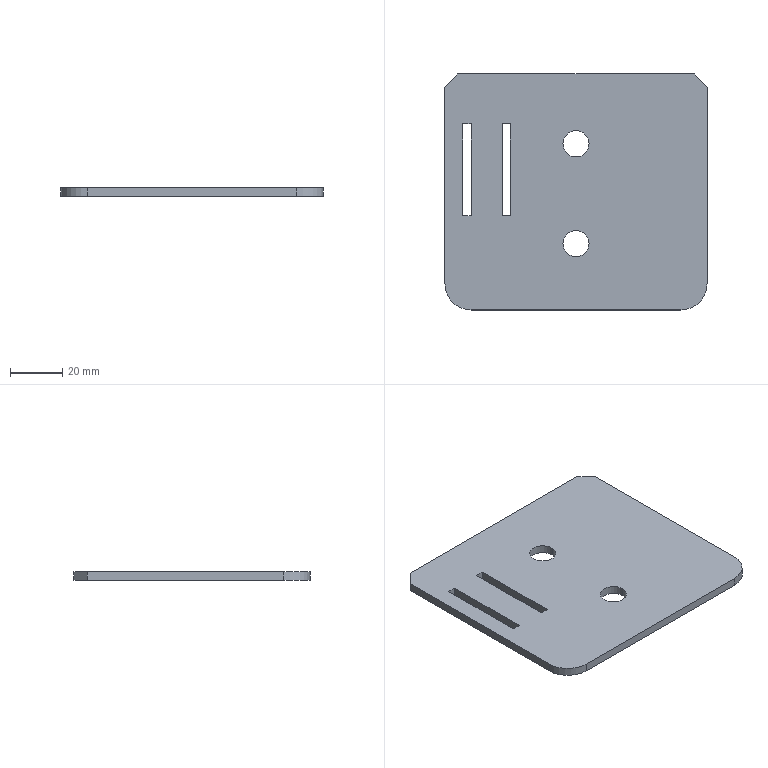Part | SolidWorks | features FlatPattern 1, SMBaseFlange 1, SheetMetal 1 | 1 solid | 22 faces | box 100 x 90 x 3.2 mm | volume 27363 mm3 | plane 16 | cylinder 6 | commonest cylinder face diameters 10 x4 20 x2
STEP:
#1=CARTESIAN_POINT('',(-190.,439.179,3.2));
#2=VERTEX_POINT('',#1);
#3=CARTESIAN_POINT('',(-180.,439.179,3.2));
#4=VERTEX_POINT('',#3);
#5=CARTESIAN_POINT('',(-185.,439.179,3.2));
#6=DIRECTION('',(0.,0.,1.));
#7=DIRECTION('',(1.,0.,0.));
#8=AXIS2_PLACEMENT_3D('',#5,#6,#7);
#9=CIRCLE('',#8,5.);
#10=EDGE_CURVE('',#2,#4,#9,.T.);
#11=ORIENTED_EDGE('',*,*,#10,.T.);
#12=CARTESIAN_POINT('',(-180.,439.179,0.));
#13=VERTEX_POINT('',#12);
#14=CARTESIAN_POINT('',(-180.,439.179,3.2));
#15=DIRECTION('',(0.,0.,-1.));
#16=VECTOR('',#15,1000.);
#17=LINE('',#14,#16);
#18=EDGE_CURVE('',#4,#13,#17,.T.);
#19=ORIENTED_EDGE('',*,*,#18,.T.);
#20=CARTESIAN_POINT('',(-190.,439.179,0.));
#21=VERTEX_POINT('',#20);
#22=CARTESIAN_POINT('',(-185.,439.179,0.));
#23=DIRECTION('',(0.,0.,1.));
#24=DIRECTION('',(1.,0.,0.));
#25=AXIS2_PLACEMENT_3D('',#22,#23,#24);
#26=CIRCLE('',#25,5.);
#27=EDGE_CURVE('',#21,#13,#26,.T.);
#28=ORIENTED_EDGE('',*,*,#27,.F.);
#29=CARTESIAN_POINT('',(-190.,439.179,3.2));
#30=DIRECTION('',(0.,0.,-1.));
#31=VECTOR('',#30,1000.);
#32=LINE('',#29,#31);
#33=EDGE_CURVE('',#2,#21,#32,.T.);
#34=ORIENTED_EDGE('',*,*,#33,.F.);
#35=EDGE_LOOP('',(#11,#19,#28,#34));
#36=FACE_OUTER_BOUND('',#35,.T.);
#37=CARTESIAN_POINT('',(-185.,439.179,3.2));
#38=DIRECTION('',(0.,0.,-1.));
#39=DIRECTION('',(-1.,0.,0.));
#40=AXIS2_PLACEMENT_3D('',#37,#38,#39);
#41=CYLINDRICAL_SURFACE('',#40,5.);
#42=ADVANCED_FACE('',(#36),#41,.F.);
#43=CARTESIAN_POINT('',(-190.,477.279,3.2));
#44=VERTEX_POINT('',#43);
#45=CARTESIAN_POINT('',(-180.,477.279,3.2));
#46=VERTEX_POINT('',#45);
#47=CARTESIAN_POINT('',(-185.,477.279,3.2));
#48=DIRECTION('',(0.,0.,1.));
#49=DIRECTION('',(1.,0.,0.));
#50=AXIS2_PLACEMENT_3D('',#47,#48,#49);
#51=CIRCLE('',#50,5.);
#52=EDGE_CURVE('',#44,#46,#51,.T.);
#53=ORIENTED_EDGE('',*,*,#52,.T.);
#54=CARTESIAN_POINT('',(-180.,477.279,0.));
#55=VERTEX_POINT('',#54);
#56=CARTESIAN_POINT('',(-180.,477.279,3.2));
#57=DIRECTION('',(0.,0.,-1.));
#58=VECTOR('',#57,1000.);
#59=LINE('',#56,#58);
#60=EDGE_CURVE('',#46,#55,#59,.T.);
#61=ORIENTED_EDGE('',*,*,#60,.T.);
#62=CARTESIAN_POINT('',(-190.,477.279,0.));
#63=VERTEX_POINT('',#62);
#64=CARTESIAN_POINT('',(-185.,477.279,0.));
#65=DIRECTION('',(0.,0.,1.));
#66=DIRECTION('',(1.,0.,0.));
#67=AXIS2_PLACEMENT_3D('',#64,#65,#66);
#68=CIRCLE('',#67,5.);
#69=EDGE_CURVE('',#63,#55,#68,.T.);
#70=ORIENTED_EDGE('',*,*,#69,.F.);
#71=CARTESIAN_POINT('',(-190.,477.279,3.2));
#72=DIRECTION('',(0.,0.,-1.));
#73=VECTOR('',#72,1000.);
#74=LINE('',#71,#73);
#75=EDGE_CURVE('',#44,#63,#74,.T.);
#76=ORIENTED_EDGE('',*,*,#75,.F.);
#77=EDGE_LOOP('',(#53,#61,#70,#76));
#78=FACE_OUTER_BOUND('',#77,.T.);
#79=CARTESIAN_POINT('',(-185.,477.279,3.2));
#80=DIRECTION('',(0.,0.,-1.));
#81=DIRECTION('',(-1.,0.,0.));
#82=AXIS2_PLACEMENT_3D('',#79,#80,#81);
#83=CYLINDRICAL_SURFACE('',#82,5.);
#84=ADVANCED_FACE('',(#78),#83,.F.);
#85=CARTESIAN_POINT('',(-228.2,484.857,3.2));
#86=VERTEX_POINT('',#85);
#87=CARTESIAN_POINT('',(-228.2,449.857,3.2));
#88=VERTEX_POINT('',#87);
#89=CARTESIAN_POINT('',(-228.2,484.857,3.2));
#90=DIRECTION('',(0.,-1.,0.));
#91=VECTOR('',#90,1000.);
#92=LINE('',#89,#91);
#93=EDGE_CURVE('',#86,#88,#92,.T.);
#94=ORIENTED_EDGE('',*,*,#93,.F.);
#95=CARTESIAN_POINT('',(-225.,484.857,3.2));
#96=VERTEX_POINT('',#95);
#97=CARTESIAN_POINT('',(-228.2,484.857,3.2));
#98=DIRECTION('',(-1.,0.,0.));
#99=VECTOR('',#98,1000.);
#100=LINE('',#97,#99);
#101=EDGE_CURVE('',#96,#86,#100,.T.);
#102=ORIENTED_EDGE('',*,*,#101,.F.);
#103=CARTESIAN_POINT('',(-225.,449.857,3.2));
#104=VERTEX_POINT('',#103);
#105=CARTESIAN_POINT('',(-225.,484.857,3.2));
#106=DIRECTION('',(0.,1.,0.));
#107=VECTOR('',#106,1000.);
#108=LINE('',#105,#107);
#109=EDGE_CURVE('',#104,#96,#108,.T.);
#110=ORIENTED_EDGE('',*,*,#109,.F.);
#111=CARTESIAN_POINT('',(-228.2,449.857,3.2));
#112=DIRECTION('',(1.,0.,0.));
#113=VECTOR('',#112,1000.);
#114=LINE('',#111,#113);
#115=EDGE_CURVE('',#88,#104,#114,.T.);
#116=ORIENTED_EDGE('',*,*,#115,.F.);
#117=EDGE_LOOP('',(#94,#102,#110,#116));
#118=FACE_BOUND('',#117,.T.);
#119=CARTESIAN_POINT('',(-230.,503.879,3.2));
#120=VERTEX_POINT('',#119);
#121=CARTESIAN_POINT('',(-235.,498.879,3.2));
#122=VERTEX_POINT('',#121);
#123=CARTESIAN_POINT('',(-235.,498.879,3.2));
#124=DIRECTION('',(-0.7071,-0.7071,0.));
#125=VECTOR('',#124,1000.);
#126=LINE('',#123,#125);
#127=EDGE_CURVE('',#120,#122,#126,.T.);
#128=ORIENTED_EDGE('',*,*,#127,.T.);
#129=CARTESIAN_POINT('',(-235.,423.879,3.2));
#130=VERTEX_POINT('',#129);
#131=CARTESIAN_POINT('',(-235.,423.879,3.2));
#132=DIRECTION('',(0.,-1.,0.));
#133=VECTOR('',#132,1000.);
#134=LINE('',#131,#133);
#135=EDGE_CURVE('',#122,#130,#134,.T.);
#136=ORIENTED_EDGE('',*,*,#135,.T.);
#137=CARTESIAN_POINT('',(-225.,413.879,3.2));
#138=VERTEX_POINT('',#137);
#139=CARTESIAN_POINT('',(-225.,423.879,3.2));
#140=DIRECTION('',(0.,0.,1.));
#141=DIRECTION('',(-1.,0.,0.));
#142=AXIS2_PLACEMENT_3D('',#139,#140,#141);
#143=CIRCLE('',#142,10.);
#144=EDGE_CURVE('',#130,#138,#143,.T.);
#145=ORIENTED_EDGE('',*,*,#144,.T.);
#146=CARTESIAN_POINT('',(-145.,413.879,3.2));
#147=VERTEX_POINT('',#146);
#148=CARTESIAN_POINT('',(-145.,413.879,3.2));
#149=DIRECTION('',(1.,0.,0.));
#150=VECTOR('',#149,1000.);
#151=LINE('',#148,#150);
#152=EDGE_CURVE('',#138,#147,#151,.T.);
#153=ORIENTED_EDGE('',*,*,#152,.T.);
#154=CARTESIAN_POINT('',(-135.,423.879,3.2));
#155=VERTEX_POINT('',#154);
#156=CARTESIAN_POINT('',(-145.,423.879,3.2));
#157=DIRECTION('',(0.,0.,1.));
#158=DIRECTION('',(-1.,0.,0.));
#159=AXIS2_PLACEMENT_3D('',#156,#157,#158);
#160=CIRCLE('',#159,10.);
#161=EDGE_CURVE('',#147,#155,#160,.T.);
#162=ORIENTED_EDGE('',*,*,#161,.T.);
#163=CARTESIAN_POINT('',(-135.,498.879,3.2));
#164=VERTEX_POINT('',#163);
#165=CARTESIAN_POINT('',(-135.,498.879,3.2));
#166=DIRECTION('',(0.,1.,0.));
#167=VECTOR('',#166,1000.);
#168=LINE('',#165,#167);
#169=EDGE_CURVE('',#155,#164,#168,.T.);
#170=ORIENTED_EDGE('',*,*,#169,.T.);
#171=CARTESIAN_POINT('',(-140.,503.879,3.2));
#172=VERTEX_POINT('',#171);
#173=CARTESIAN_POINT('',(-140.,503.879,3.2));
#174=DIRECTION('',(-0.7071,0.7071,0.));
#175=VECTOR('',#174,1000.);
#176=LINE('',#173,#175);
#177=EDGE_CURVE('',#164,#172,#176,.T.);
#178=ORIENTED_EDGE('',*,*,#177,.T.);
#179=CARTESIAN_POINT('',(-230.,503.879,3.2));
#180=DIRECTION('',(-1.,0.,0.));
#181=VECTOR('',#180,1000.);
#182=LINE('',#179,#181);
#183=EDGE_CURVE('',#172,#120,#182,.T.);
#184=ORIENTED_EDGE('',*,*,#183,.T.);
#185=EDGE_LOOP('',(#128,#136,#145,#153,#162,#170,#178,#184));
#186=FACE_OUTER_BOUND('',#185,.T.);
#187=ORIENTED_EDGE('',*,*,#52,.F.);
#188=CARTESIAN_POINT('',(-185.,477.279,3.2));
#189=DIRECTION('',(0.,0.,1.));
#190=DIRECTION('',(1.,0.,0.));
#191=AXIS2_PLACEMENT_3D('',#188,#189,#190);
#192=CIRCLE('',#191,5.);
#193=EDGE_CURVE('',#46,#44,#192,.T.);
#194=ORIENTED_EDGE('',*,*,#193,.F.);
#195=EDGE_LOOP('',(#187,#194));
#196=FACE_BOUND('',#195,.T.);
#197=ORIENTED_EDGE('',*,*,#10,.F.);
#198=CARTESIAN_POINT('',(-185.,439.179,3.2));
#199=DIRECTION('',(0.,0.,1.));
#200=DIRECTION('',(1.,0.,0.));
#201=AXIS2_PLACEMENT_3D('',#198,#199,#200);
#202=CIRCLE('',#201,5.);
#203=EDGE_CURVE('',#4,#2,#202,.T.);
#204=ORIENTED_EDGE('',*,*,#203,.F.);
#205=EDGE_LOOP('',(#197,#204));
#206=FACE_BOUND('',#205,.T.);
#207=CARTESIAN_POINT('',(-213.2,484.857,3.2));
#208=VERTEX_POINT('',#207);
#209=CARTESIAN_POINT('',(-213.2,449.857,3.2));
#210=VERTEX_POINT('',#209);
#211=CARTESIAN_POINT('',(-213.2,484.857,3.2));
#212=DIRECTION('',(0.,-1.,0.));
#213=VECTOR('',#212,1000.);
#214=LINE('',#211,#213);
#215=EDGE_CURVE('',#208,#210,#214,.T.);
#216=ORIENTED_EDGE('',*,*,#215,.F.);
#217=CARTESIAN_POINT('',(-210.,484.857,3.2));
#218=VERTEX_POINT('',#217);
#219=CARTESIAN_POINT('',(-213.2,484.857,3.2));
#220=DIRECTION('',(-1.,0.,0.));
#221=VECTOR('',#220,1000.);
#222=LINE('',#219,#221);
#223=EDGE_CURVE('',#218,#208,#222,.T.);
#224=ORIENTED_EDGE('',*,*,#223,.F.);
#225=CARTESIAN_POINT('',(-210.,449.857,3.2));
#226=VERTEX_POINT('',#225);
#227=CARTESIAN_POINT('',(-210.,484.857,3.2));
#228=DIRECTION('',(0.,1.,0.));
#229=VECTOR('',#228,1000.);
#230=LINE('',#227,#229);
#231=EDGE_CURVE('',#226,#218,#230,.T.);
#232=ORIENTED_EDGE('',*,*,#231,.F.);
#233=CARTESIAN_POINT('',(-213.2,449.857,3.2));
#234=DIRECTION('',(1.,0.,0.));
#235=VECTOR('',#234,1000.);
#236=LINE('',#233,#235);
#237=EDGE_CURVE('',#210,#226,#236,.T.);
#238=ORIENTED_EDGE('',*,*,#237,.F.);
#239=EDGE_LOOP('',(#216,#224,#232,#238));
#240=FACE_BOUND('',#239,.T.);
#241=CARTESIAN_POINT('',(-145.,423.879,3.2));
#242=DIRECTION('',(0.,0.,-1.));
#243=DIRECTION('',(-1.,0.,0.));
#244=AXIS2_PLACEMENT_3D('',#241,#242,#243);
#245=PLANE('',#244);
#246=ADVANCED_FACE('',(#118,#186,#196,#206,#240),#245,.F.);
#247=ORIENTED_EDGE('',*,*,#69,.T.);
#248=CARTESIAN_POINT('',(-185.,477.279,0.));
#249=DIRECTION('',(0.,0.,1.));
#250=DIRECTION('',(1.,0.,0.));
#251=AXIS2_PLACEMENT_3D('',#248,#249,#250);
#252=CIRCLE('',#251,5.);
#253=EDGE_CURVE('',#55,#63,#252,.T.);
#254=ORIENTED_EDGE('',*,*,#253,.T.);
#255=EDGE_LOOP('',(#247,#254));
#256=FACE_BOUND('',#255,.T.);
#257=CARTESIAN_POINT('',(-230.,503.879,0.));
#258=VERTEX_POINT('',#257);
#259=CARTESIAN_POINT('',(-235.,498.879,0.));
#260=VERTEX_POINT('',#259);
#261=CARTESIAN_POINT('',(-235.,498.879,0.));
#262=DIRECTION('',(-0.7071,-0.7071,0.));
#263=VECTOR('',#262,1000.);
#264=LINE('',#261,#263);
#265=EDGE_CURVE('',#258,#260,#264,.T.);
#266=ORIENTED_EDGE('',*,*,#265,.F.);
#267=CARTESIAN_POINT('',(-140.,503.879,0.));
#268=VERTEX_POINT('',#267);
#269=CARTESIAN_POINT('',(-230.,503.879,0.));
#270=DIRECTION('',(-1.,0.,0.));
#271=VECTOR('',#270,1000.);
#272=LINE('',#269,#271);
#273=EDGE_CURVE('',#268,#258,#272,.T.);
#274=ORIENTED_EDGE('',*,*,#273,.F.);
#275=CARTESIAN_POINT('',(-135.,498.879,0.));
#276=VERTEX_POINT('',#275);
#277=CARTESIAN_POINT('',(-140.,503.879,0.));
#278=DIRECTION('',(-0.7071,0.7071,0.));
#279=VECTOR('',#278,1000.);
#280=LINE('',#277,#279);
#281=EDGE_CURVE('',#276,#268,#280,.T.);
#282=ORIENTED_EDGE('',*,*,#281,.F.);
#283=CARTESIAN_POINT('',(-135.,423.879,0.));
#284=VERTEX_POINT('',#283);
#285=CARTESIAN_POINT('',(-135.,498.879,0.));
#286=DIRECTION('',(0.,1.,0.));
#287=VECTOR('',#286,1000.);
#288=LINE('',#285,#287);
#289=EDGE_CURVE('',#284,#276,#288,.T.);
#290=ORIENTED_EDGE('',*,*,#289,.F.);
#291=CARTESIAN_POINT('',(-145.,413.879,0.));
#292=VERTEX_POINT('',#291);
#293=CARTESIAN_POINT('',(-145.,423.879,0.));
#294=DIRECTION('',(0.,0.,1.));
#295=DIRECTION('',(-1.,0.,0.));
#296=AXIS2_PLACEMENT_3D('',#293,#294,#295);
#297=CIRCLE('',#296,10.);
#298=EDGE_CURVE('',#292,#284,#297,.T.);
#299=ORIENTED_EDGE('',*,*,#298,.F.);
#300=CARTESIAN_POINT('',(-225.,413.879,0.));
#301=VERTEX_POINT('',#300);
#302=CARTESIAN_POINT('',(-145.,413.879,0.));
#303=DIRECTION('',(1.,0.,0.));
#304=VECTOR('',#303,1000.);
#305=LINE('',#302,#304);
#306=EDGE_CURVE('',#301,#292,#305,.T.);
#307=ORIENTED_EDGE('',*,*,#306,.F.);
#308=CARTESIAN_POINT('',(-235.,423.879,0.));
#309=VERTEX_POINT('',#308);
#310=CARTESIAN_POINT('',(-225.,423.879,0.));
#311=DIRECTION('',(0.,0.,1.));
#312=DIRECTION('',(-1.,0.,0.));
#313=AXIS2_PLACEMENT_3D('',#310,#311,#312);
#314=CIRCLE('',#313,10.);
#315=EDGE_CURVE('',#309,#301,#314,.T.);
#316=ORIENTED_EDGE('',*,*,#315,.F.);
#317=CARTESIAN_POINT('',(-235.,423.879,0.));
#318=DIRECTION('',(0.,-1.,0.));
#319=VECTOR('',#318,1000.);
#320=LINE('',#317,#319);
#321=EDGE_CURVE('',#260,#309,#320,.T.);
#322=ORIENTED_EDGE('',*,*,#321,.F.);
#323=EDGE_LOOP('',(#266,#274,#282,#290,#299,#307,#316,#322));
#324=FACE_OUTER_BOUND('',#323,.T.);
#325=ORIENTED_EDGE('',*,*,#27,.T.);
#326=CARTESIAN_POINT('',(-185.,439.179,0.));
#327=DIRECTION('',(0.,0.,1.));
#328=DIRECTION('',(1.,0.,0.));
#329=AXIS2_PLACEMENT_3D('',#326,#327,#328);
#330=CIRCLE('',#329,5.);
#331=EDGE_CURVE('',#13,#21,#330,.T.);
#332=ORIENTED_EDGE('',*,*,#331,.T.);
#333=EDGE_LOOP('',(#325,#332));
#334=FACE_BOUND('',#333,.T.);
#335=CARTESIAN_POINT('',(-225.,484.857,0.));
#336=VERTEX_POINT('',#335);
#337=CARTESIAN_POINT('',(-228.2,484.857,0.));
#338=VERTEX_POINT('',#337);
#339=CARTESIAN_POINT('',(-228.2,484.857,0.));
#340=DIRECTION('',(-1.,0.,0.));
#341=VECTOR('',#340,1000.);
#342=LINE('',#339,#341);
#343=EDGE_CURVE('',#336,#338,#342,.T.);
#344=ORIENTED_EDGE('',*,*,#343,.T.);
#345=CARTESIAN_POINT('',(-228.2,449.857,0.));
#346=VERTEX_POINT('',#345);
#347=CARTESIAN_POINT('',(-228.2,484.857,0.));
#348=DIRECTION('',(0.,-1.,0.));
#349=VECTOR('',#348,1000.);
#350=LINE('',#347,#349);
#351=EDGE_CURVE('',#338,#346,#350,.T.);
#352=ORIENTED_EDGE('',*,*,#351,.T.);
#353=CARTESIAN_POINT('',(-225.,449.857,0.));
#354=VERTEX_POINT('',#353);
#355=CARTESIAN_POINT('',(-228.2,449.857,0.));
#356=DIRECTION('',(1.,0.,0.));
#357=VECTOR('',#356,1000.);
#358=LINE('',#355,#357);
#359=EDGE_CURVE('',#346,#354,#358,.T.);
#360=ORIENTED_EDGE('',*,*,#359,.T.);
#361=CARTESIAN_POINT('',(-225.,484.857,0.));
#362=DIRECTION('',(0.,1.,0.));
#363=VECTOR('',#362,1000.);
#364=LINE('',#361,#363);
#365=EDGE_CURVE('',#354,#336,#364,.T.);
#366=ORIENTED_EDGE('',*,*,#365,.T.);
#367=EDGE_LOOP('',(#344,#352,#360,#366));
#368=FACE_BOUND('',#367,.T.);
#369=CARTESIAN_POINT('',(-210.,484.857,0.));
#370=VERTEX_POINT('',#369);
#371=CARTESIAN_POINT('',(-213.2,484.857,0.));
#372=VERTEX_POINT('',#371);
#373=CARTESIAN_POINT('',(-213.2,484.857,0.));
#374=DIRECTION('',(-1.,0.,0.));
#375=VECTOR('',#374,1000.);
#376=LINE('',#373,#375);
#377=EDGE_CURVE('',#370,#372,#376,.T.);
#378=ORIENTED_EDGE('',*,*,#377,.T.);
#379=CARTESIAN_POINT('',(-213.2,449.857,0.));
#380=VERTEX_POINT('',#379);
#381=CARTESIAN_POINT('',(-213.2,484.857,0.));
#382=DIRECTION('',(0.,-1.,0.));
#383=VECTOR('',#382,1000.);
#384=LINE('',#381,#383);
#385=EDGE_CURVE('',#372,#380,#384,.T.);
#386=ORIENTED_EDGE('',*,*,#385,.T.);
#387=CARTESIAN_POINT('',(-210.,449.857,0.));
#388=VERTEX_POINT('',#387);
#389=CARTESIAN_POINT('',(-213.2,449.857,0.));
#390=DIRECTION('',(1.,0.,0.));
#391=VECTOR('',#390,1000.);
#392=LINE('',#389,#391);
#393=EDGE_CURVE('',#380,#388,#392,.T.);
#394=ORIENTED_EDGE('',*,*,#393,.T.);
#395=CARTESIAN_POINT('',(-210.,484.857,0.));
#396=DIRECTION('',(0.,1.,0.));
#397=VECTOR('',#396,1000.);
#398=LINE('',#395,#397);
#399=EDGE_CURVE('',#388,#370,#398,.T.);
#400=ORIENTED_EDGE('',*,*,#399,.T.);
#401=EDGE_LOOP('',(#378,#386,#394,#400));
#402=FACE_BOUND('',#401,.T.);
#403=CARTESIAN_POINT('',(-145.,423.879,0.));
#404=DIRECTION('',(0.,0.,-1.));
#405=DIRECTION('',(-1.,0.,0.));
#406=AXIS2_PLACEMENT_3D('',#403,#404,#405);
#407=PLANE('',#406);
#408=ADVANCED_FACE('',(#256,#324,#334,#368,#402),#407,.T.);
#409=ORIENTED_EDGE('',*,*,#265,.T.);
#410=CARTESIAN_POINT('',(-235.,498.879,3.2));
#411=DIRECTION('',(0.,0.,-1.));
#412=VECTOR('',#411,1000.);
#413=LINE('',#410,#412);
#414=EDGE_CURVE('',#122,#260,#413,.T.);
#415=ORIENTED_EDGE('',*,*,#414,.F.);
#416=ORIENTED_EDGE('',*,*,#127,.F.);
#417=CARTESIAN_POINT('',(-230.,503.879,3.2));
#418=DIRECTION('',(0.,0.,-1.));
#419=VECTOR('',#418,1000.);
#420=LINE('',#417,#419);
#421=EDGE_CURVE('',#120,#258,#420,.T.);
#422=ORIENTED_EDGE('',*,*,#421,.T.);
#423=EDGE_LOOP('',(#409,#415,#416,#422));
#424=FACE_OUTER_BOUND('',#423,.T.);
#425=CARTESIAN_POINT('',(-235.,498.879,3.2));
#426=DIRECTION('',(0.7071,-0.7071,0.));
#427=DIRECTION('',(0.7071,0.7071,0.));
#428=AXIS2_PLACEMENT_3D('',#425,#426,#427);
#429=PLANE('',#428);
#430=ADVANCED_FACE('',(#424),#429,.F.);
#431=ORIENTED_EDGE('',*,*,#321,.T.);
#432=CARTESIAN_POINT('',(-235.,423.879,3.2));
#433=DIRECTION('',(0.,0.,-1.));
#434=VECTOR('',#433,1000.);
#435=LINE('',#432,#434);
#436=EDGE_CURVE('',#130,#309,#435,.T.);
#437=ORIENTED_EDGE('',*,*,#436,.F.);
#438=ORIENTED_EDGE('',*,*,#135,.F.);
#439=ORIENTED_EDGE('',*,*,#414,.T.);
#440=EDGE_LOOP('',(#431,#437,#438,#439));
#441=FACE_OUTER_BOUND('',#440,.T.);
#442=CARTESIAN_POINT('',(-235.,423.879,3.2));
#443=DIRECTION('',(1.,0.,0.));
#444=DIRECTION('',(0.,0.,-1.));
#445=AXIS2_PLACEMENT_3D('',#442,#443,#444);
#446=PLANE('',#445);
#447=ADVANCED_FACE('',(#441),#446,.F.);
#448=ORIENTED_EDGE('',*,*,#315,.T.);
#449=CARTESIAN_POINT('',(-225.,413.879,3.2));
#450=DIRECTION('',(0.,0.,-1.));
#451=VECTOR('',#450,1000.);
#452=LINE('',#449,#451);
#453=EDGE_CURVE('',#138,#301,#452,.T.);
#454=ORIENTED_EDGE('',*,*,#453,.F.);
#455=ORIENTED_EDGE('',*,*,#144,.F.);
#456=ORIENTED_EDGE('',*,*,#436,.T.);
#457=EDGE_LOOP('',(#448,#454,#455,#456));
#458=FACE_OUTER_BOUND('',#457,.T.);
#459=CARTESIAN_POINT('',(-225.,423.879,3.2));
#460=DIRECTION('',(0.,0.,-1.));
#461=DIRECTION('',(-1.,0.,0.));
#462=AXIS2_PLACEMENT_3D('',#459,#460,#461);
#463=CYLINDRICAL_SURFACE('',#462,10.);
#464=ADVANCED_FACE('',(#458),#463,.T.);
#465=ORIENTED_EDGE('',*,*,#306,.T.);
#466=CARTESIAN_POINT('',(-145.,413.879,3.2));
#467=DIRECTION('',(0.,0.,-1.));
#468=VECTOR('',#467,1000.);
#469=LINE('',#466,#468);
#470=EDGE_CURVE('',#147,#292,#469,.T.);
#471=ORIENTED_EDGE('',*,*,#470,.F.);
#472=ORIENTED_EDGE('',*,*,#152,.F.);
#473=ORIENTED_EDGE('',*,*,#453,.T.);
#474=EDGE_LOOP('',(#465,#471,#472,#473));
#475=FACE_OUTER_BOUND('',#474,.T.);
#476=CARTESIAN_POINT('',(-145.,413.879,3.2));
#477=DIRECTION('',(0.,1.,0.));
#478=DIRECTION('',(0.,0.,1.));
#479=AXIS2_PLACEMENT_3D('',#476,#477,#478);
#480=PLANE('',#479);
#481=ADVANCED_FACE('',(#475),#480,.F.);
#482=ORIENTED_EDGE('',*,*,#298,.T.);
#483=CARTESIAN_POINT('',(-135.,423.879,3.2));
#484=DIRECTION('',(0.,0.,-1.));
#485=VECTOR('',#484,1000.);
#486=LINE('',#483,#485);
#487=EDGE_CURVE('',#155,#284,#486,.T.);
#488=ORIENTED_EDGE('',*,*,#487,.F.);
#489=ORIENTED_EDGE('',*,*,#161,.F.);
#490=ORIENTED_EDGE('',*,*,#470,.T.);
#491=EDGE_LOOP('',(#482,#488,#489,#490));
#492=FACE_OUTER_BOUND('',#491,.T.);
#493=CARTESIAN_POINT('',(-145.,423.879,3.2));
#494=DIRECTION('',(0.,0.,-1.));
#495=DIRECTION('',(-1.,0.,0.));
#496=AXIS2_PLACEMENT_3D('',#493,#494,#495);
#497=CYLINDRICAL_SURFACE('',#496,10.);
#498=ADVANCED_FACE('',(#492),#497,.T.);
#499=ORIENTED_EDGE('',*,*,#289,.T.);
#500=CARTESIAN_POINT('',(-135.,498.879,3.2));
#501=DIRECTION('',(0.,0.,-1.));
#502=VECTOR('',#501,1000.);
#503=LINE('',#500,#502);
#504=EDGE_CURVE('',#164,#276,#503,.T.);
#505=ORIENTED_EDGE('',*,*,#504,.F.);
#506=ORIENTED_EDGE('',*,*,#169,.F.);
#507=ORIENTED_EDGE('',*,*,#487,.T.);
#508=EDGE_LOOP('',(#499,#505,#506,#507));
#509=FACE_OUTER_BOUND('',#508,.T.);
#510=CARTESIAN_POINT('',(-135.,498.879,3.2));
#511=DIRECTION('',(-1.,0.,0.));
#512=DIRECTION('',(0.,0.,1.));
#513=AXIS2_PLACEMENT_3D('',#510,#511,#512);
#514=PLANE('',#513);
#515=ADVANCED_FACE('',(#509),#514,.F.);
#516=ORIENTED_EDGE('',*,*,#281,.T.);
#517=CARTESIAN_POINT('',(-140.,503.879,3.2));
#518=DIRECTION('',(0.,0.,-1.));
#519=VECTOR('',#518,1000.);
#520=LINE('',#517,#519);
#521=EDGE_CURVE('',#172,#268,#520,.T.);
#522=ORIENTED_EDGE('',*,*,#521,.F.);
#523=ORIENTED_EDGE('',*,*,#177,.F.);
#524=ORIENTED_EDGE('',*,*,#504,.T.);
#525=EDGE_LOOP('',(#516,#522,#523,#524));
#526=FACE_OUTER_BOUND('',#525,.T.);
#527=CARTESIAN_POINT('',(-140.,503.879,3.2));
#528=DIRECTION('',(-0.7071,-0.7071,0.));
#529=DIRECTION('',(0.7071,-0.7071,0.));
#530=AXIS2_PLACEMENT_3D('',#527,#528,#529);
#531=PLANE('',#530);
#532=ADVANCED_FACE('',(#526),#531,.F.);
#533=ORIENTED_EDGE('',*,*,#273,.T.);
#534=ORIENTED_EDGE('',*,*,#421,.F.);
#535=ORIENTED_EDGE('',*,*,#183,.F.);
#536=ORIENTED_EDGE('',*,*,#521,.T.);
#537=EDGE_LOOP('',(#533,#534,#535,#536));
#538=FACE_OUTER_BOUND('',#537,.T.);
#539=CARTESIAN_POINT('',(-230.,503.879,3.2));
#540=DIRECTION('',(0.,-1.,0.));
#541=DIRECTION('',(1.,0.,0.));
#542=AXIS2_PLACEMENT_3D('',#539,#540,#541);
#543=PLANE('',#542);
#544=ADVANCED_FACE('',(#538),#543,.F.);
#545=ORIENTED_EDGE('',*,*,#60,.F.);
#546=ORIENTED_EDGE('',*,*,#193,.T.);
#547=ORIENTED_EDGE('',*,*,#75,.T.);
#548=ORIENTED_EDGE('',*,*,#253,.F.);
#549=EDGE_LOOP('',(#545,#546,#547,#548));
#550=FACE_OUTER_BOUND('',#549,.T.);
#551=CARTESIAN_POINT('',(-185.,477.279,3.2));
#552=DIRECTION('',(0.,0.,-1.));
#553=DIRECTION('',(-1.,0.,0.));
#554=AXIS2_PLACEMENT_3D('',#551,#552,#553);
#555=CYLINDRICAL_SURFACE('',#554,5.);
#556=ADVANCED_FACE('',(#550),#555,.F.);
#557=ORIENTED_EDGE('',*,*,#18,.F.);
#558=ORIENTED_EDGE('',*,*,#203,.T.);
#559=ORIENTED_EDGE('',*,*,#33,.T.);
#560=ORIENTED_EDGE('',*,*,#331,.F.);
#561=EDGE_LOOP('',(#557,#558,#559,#560));
#562=FACE_OUTER_BOUND('',#561,.T.);
#563=CARTESIAN_POINT('',(-185.,439.179,3.2));
#564=DIRECTION('',(0.,0.,-1.));
#565=DIRECTION('',(-1.,0.,0.));
#566=AXIS2_PLACEMENT_3D('',#563,#564,#565);
#567=CYLINDRICAL_SURFACE('',#566,5.);
#568=ADVANCED_FACE('',(#562),#567,.F.);
#569=ORIENTED_EDGE('',*,*,#351,.F.);
#570=CARTESIAN_POINT('',(-228.2,484.857,3.2));
#571=DIRECTION('',(0.,0.,-1.));
#572=VECTOR('',#571,1000.);
#573=LINE('',#570,#572);
#574=EDGE_CURVE('',#86,#338,#573,.T.);
#575=ORIENTED_EDGE('',*,*,#574,.F.);
#576=ORIENTED_EDGE('',*,*,#93,.T.);
#577=CARTESIAN_POINT('',(-228.2,449.857,3.2));
#578=DIRECTION('',(0.,0.,-1.));
#579=VECTOR('',#578,1000.);
#580=LINE('',#577,#579);
#581=EDGE_CURVE('',#88,#346,#580,.T.);
#582=ORIENTED_EDGE('',*,*,#581,.T.);
#583=EDGE_LOOP('',(#569,#575,#576,#582));
#584=FACE_OUTER_BOUND('',#583,.T.);
#585=CARTESIAN_POINT('',(-228.2,484.857,3.2));
#586=DIRECTION('',(1.,0.,0.));
#587=DIRECTION('',(0.,0.,-1.));
#588=AXIS2_PLACEMENT_3D('',#585,#586,#587);
#589=PLANE('',#588);
#590=ADVANCED_FACE('',(#584),#589,.T.);
#591=ORIENTED_EDGE('',*,*,#359,.F.);
#592=ORIENTED_EDGE('',*,*,#581,.F.);
#593=ORIENTED_EDGE('',*,*,#115,.T.);
#594=CARTESIAN_POINT('',(-225.,449.857,3.2));
#595=DIRECTION('',(0.,0.,-1.));
#596=VECTOR('',#595,1000.);
#597=LINE('',#594,#596);
#598=EDGE_CURVE('',#104,#354,#597,.T.);
#599=ORIENTED_EDGE('',*,*,#598,.T.);
#600=EDGE_LOOP('',(#591,#592,#593,#599));
#601=FACE_OUTER_BOUND('',#600,.T.);
#602=CARTESIAN_POINT('',(-228.2,449.857,3.2));
#603=DIRECTION('',(0.,1.,0.));
#604=DIRECTION('',(0.,0.,1.));
#605=AXIS2_PLACEMENT_3D('',#602,#603,#604);
#606=PLANE('',#605);
#607=ADVANCED_FACE('',(#601),#606,.T.);
#608=ORIENTED_EDGE('',*,*,#365,.F.);
#609=ORIENTED_EDGE('',*,*,#598,.F.);
#610=ORIENTED_EDGE('',*,*,#109,.T.);
#611=CARTESIAN_POINT('',(-225.,484.857,3.2));
#612=DIRECTION('',(0.,0.,-1.));
#613=VECTOR('',#612,1000.);
#614=LINE('',#611,#613);
#615=EDGE_CURVE('',#96,#336,#614,.T.);
#616=ORIENTED_EDGE('',*,*,#615,.T.);
#617=EDGE_LOOP('',(#608,#609,#610,#616));
#618=FACE_OUTER_BOUND('',#617,.T.);
#619=CARTESIAN_POINT('',(-225.,484.857,3.2));
#620=DIRECTION('',(-1.,0.,0.));
#621=DIRECTION('',(0.,0.,1.));
#622=AXIS2_PLACEMENT_3D('',#619,#620,#621);
#623=PLANE('',#622);
#624=ADVANCED_FACE('',(#618),#623,.T.);
#625=ORIENTED_EDGE('',*,*,#343,.F.);
#626=ORIENTED_EDGE('',*,*,#615,.F.);
#627=ORIENTED_EDGE('',*,*,#101,.T.);
#628=ORIENTED_EDGE('',*,*,#574,.T.);
#629=EDGE_LOOP('',(#625,#626,#627,#628));
#630=FACE_OUTER_BOUND('',#629,.T.);
#631=CARTESIAN_POINT('',(-228.2,484.857,3.2));
#632=DIRECTION('',(0.,-1.,0.));
#633=DIRECTION('',(0.,0.,-1.));
#634=AXIS2_PLACEMENT_3D('',#631,#632,#633);
#635=PLANE('',#634);
#636=ADVANCED_FACE('',(#630),#635,.T.);
#637=ORIENTED_EDGE('',*,*,#385,.F.);
#638=CARTESIAN_POINT('',(-213.2,484.857,3.2));
#639=DIRECTION('',(0.,0.,-1.));
#640=VECTOR('',#639,1000.);
#641=LINE('',#638,#640);
#642=EDGE_CURVE('',#208,#372,#641,.T.);
#643=ORIENTED_EDGE('',*,*,#642,.F.);
#644=ORIENTED_EDGE('',*,*,#215,.T.);
#645=CARTESIAN_POINT('',(-213.2,449.857,3.2));
#646=DIRECTION('',(0.,0.,-1.));
#647=VECTOR('',#646,1000.);
#648=LINE('',#645,#647);
#649=EDGE_CURVE('',#210,#380,#648,.T.);
#650=ORIENTED_EDGE('',*,*,#649,.T.);
#651=EDGE_LOOP('',(#637,#643,#644,#650));
#652=FACE_OUTER_BOUND('',#651,.T.);
#653=CARTESIAN_POINT('',(-213.2,484.857,3.2));
#654=DIRECTION('',(1.,0.,0.));
#655=DIRECTION('',(0.,0.,-1.));
#656=AXIS2_PLACEMENT_3D('',#653,#654,#655);
#657=PLANE('',#656);
#658=ADVANCED_FACE('',(#652),#657,.T.);
#659=ORIENTED_EDGE('',*,*,#393,.F.);
#660=ORIENTED_EDGE('',*,*,#649,.F.);
#661=ORIENTED_EDGE('',*,*,#237,.T.);
#662=CARTESIAN_POINT('',(-210.,449.857,3.2));
#663=DIRECTION('',(0.,0.,-1.));
#664=VECTOR('',#663,1000.);
#665=LINE('',#662,#664);
#666=EDGE_CURVE('',#226,#388,#665,.T.);
#667=ORIENTED_EDGE('',*,*,#666,.T.);
#668=EDGE_LOOP('',(#659,#660,#661,#667));
#669=FACE_OUTER_BOUND('',#668,.T.);
#670=CARTESIAN_POINT('',(-213.2,449.857,3.2));
#671=DIRECTION('',(0.,1.,0.));
#672=DIRECTION('',(0.,0.,1.));
#673=AXIS2_PLACEMENT_3D('',#670,#671,#672);
#674=PLANE('',#673);
#675=ADVANCED_FACE('',(#669),#674,.T.);
#676=ORIENTED_EDGE('',*,*,#399,.F.);
#677=ORIENTED_EDGE('',*,*,#666,.F.);
#678=ORIENTED_EDGE('',*,*,#231,.T.);
#679=CARTESIAN_POINT('',(-210.,484.857,3.2));
#680=DIRECTION('',(0.,0.,-1.));
#681=VECTOR('',#680,1000.);
#682=LINE('',#679,#681);
#683=EDGE_CURVE('',#218,#370,#682,.T.);
#684=ORIENTED_EDGE('',*,*,#683,.T.);
#685=EDGE_LOOP('',(#676,#677,#678,#684));
#686=FACE_OUTER_BOUND('',#685,.T.);
#687=CARTESIAN_POINT('',(-210.,484.857,3.2));
#688=DIRECTION('',(-1.,0.,0.));
#689=DIRECTION('',(0.,0.,1.));
#690=AXIS2_PLACEMENT_3D('',#687,#688,#689);
#691=PLANE('',#690);
#692=ADVANCED_FACE('',(#686),#691,.T.);
#693=ORIENTED_EDGE('',*,*,#377,.F.);
#694=ORIENTED_EDGE('',*,*,#683,.F.);
#695=ORIENTED_EDGE('',*,*,#223,.T.);
#696=ORIENTED_EDGE('',*,*,#642,.T.);
#697=EDGE_LOOP('',(#693,#694,#695,#696));
#698=FACE_OUTER_BOUND('',#697,.T.);
#699=CARTESIAN_POINT('',(-213.2,484.857,3.2));
#700=DIRECTION('',(0.,-1.,0.));
#701=DIRECTION('',(0.,0.,-1.));
#702=AXIS2_PLACEMENT_3D('',#699,#700,#701);
#703=PLANE('',#702);
#704=ADVANCED_FACE('',(#698),#703,.T.);
#705=CLOSED_SHELL('',(#42,#84,#246,#408,#430,#447,#464,#481,#498,#515,#532,#544,#556,#568,#590,#607,#624,#636,#658,#675,#692,#704));
#706=MANIFOLD_SOLID_BREP('',#705);
#707=CARTESIAN_POINT('',(0.,0.,0.));
#708=DIRECTION('',(0.,0.,1.));
#709=DIRECTION('',(1.,0.,0.));
#710=AXIS2_PLACEMENT_3D('',#707,#708,#709);
#711=(LENGTH_UNIT()NAMED_UNIT(*)SI_UNIT(.MILLI.,.METRE.));
#712=UNCERTAINTY_MEASURE_WITH_UNIT(LENGTH_MEASURE(0.00001),#711,'','');
#713=(NAMED_UNIT(*)PLANE_ANGLE_UNIT()SI_UNIT($,.RADIAN.));
#714=(NAMED_UNIT(*)SI_UNIT($,.STERADIAN.)SOLID_ANGLE_UNIT());
#715=(GEOMETRIC_REPRESENTATION_CONTEXT(3)GLOBAL_UNCERTAINTY_ASSIGNED_CONTEXT((#712))GLOBAL_UNIT_ASSIGNED_CONTEXT((#711,#713,#714))REPRESENTATION_CONTEXT('',''));
#716=ADVANCED_BREP_SHAPE_REPRESENTATION('',(#706,#710),#715);